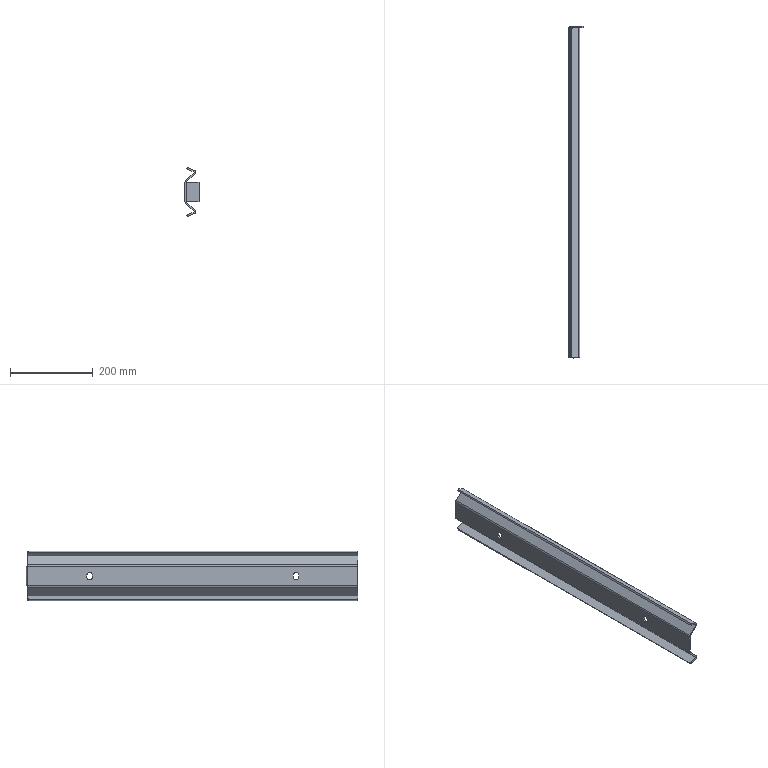Part | SolidWorks | 1 solid | 60 faces | box 34 x 804 x 120.238 mm | volume 511930 mm3 | plane 40 | cylinder 20 | commonest cylinder face diameters 10 x6 13 x6 0.2 x3 8.2 x3 2 x2